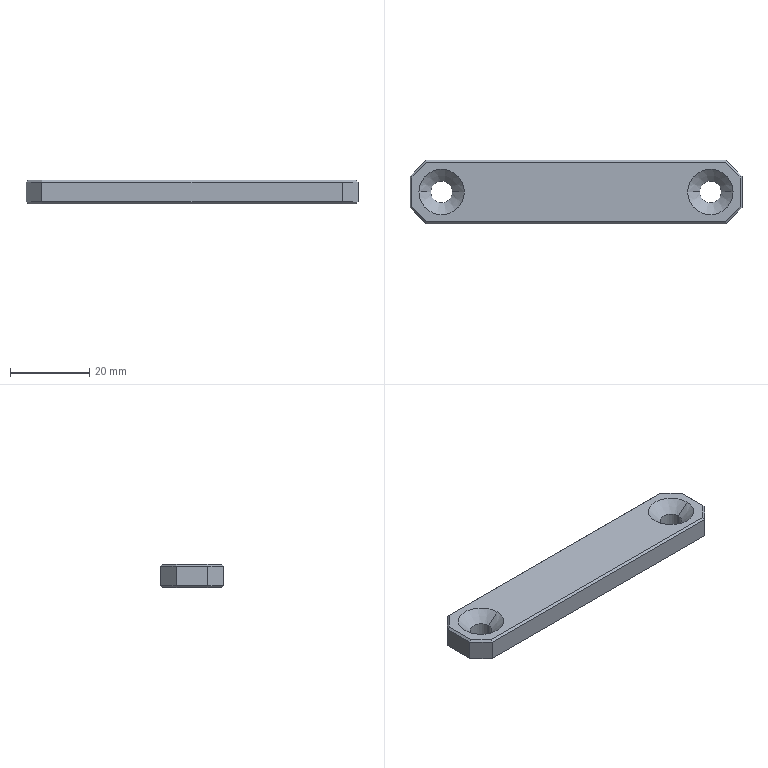Part | Creo | 1 solid | 34 faces | box 84 x 16 x 5.998 mm | volume 7341 mm3 | plane 26 | cylinder 4 | cone 4 | commonest cylinder face diameters 5.5 x4
STEP:
#1=CARTESIAN_POINT('',(-206.793,218.496,285.));
#2=VERTEX_POINT('',#1);
#3=CARTESIAN_POINT('',(-210.5,214.789,285.));
#4=VERTEX_POINT('',#3);
#5=CARTESIAN_POINT('',(-206.793,218.496,285.));
#6=DIRECTION('',(-0.7071,-0.7071,0.));
#7=VECTOR('',#6,5.243);
#8=LINE('',#5,#7);
#9=EDGE_CURVE('',#2,#4,#8,.T.);
#10=ORIENTED_EDGE('',*,*,#9,.F.);
#11=CARTESIAN_POINT('',(-131.207,218.496,285.));
#12=VERTEX_POINT('',#11);
#13=CARTESIAN_POINT('',(-206.793,218.496,285.));
#14=DIRECTION('',(1.,0.,0.));
#15=VECTOR('',#14,75.586);
#16=LINE('',#13,#15);
#17=EDGE_CURVE('',#2,#12,#16,.T.);
#18=ORIENTED_EDGE('',*,*,#17,.T.);
#19=CARTESIAN_POINT('',(-127.5,214.789,285.));
#20=VERTEX_POINT('',#19);
#21=CARTESIAN_POINT('',(-127.5,214.789,285.));
#22=DIRECTION('',(-0.7071,0.7071,0.));
#23=VECTOR('',#22,5.243);
#24=LINE('',#21,#23);
#25=EDGE_CURVE('',#20,#12,#24,.T.);
#26=ORIENTED_EDGE('',*,*,#25,.F.);
#27=CARTESIAN_POINT('',(-127.5,207.203,285.));
#28=VERTEX_POINT('',#27);
#29=CARTESIAN_POINT('',(-127.5,214.789,285.));
#30=DIRECTION('',(0.,-1.,0.));
#31=VECTOR('',#30,7.586);
#32=LINE('',#29,#31);
#33=EDGE_CURVE('',#20,#28,#32,.T.);
#34=ORIENTED_EDGE('',*,*,#33,.T.);
#35=CARTESIAN_POINT('',(-131.207,203.496,285.));
#36=VERTEX_POINT('',#35);
#37=CARTESIAN_POINT('',(-131.207,203.496,285.));
#38=DIRECTION('',(0.7071,0.7071,0.));
#39=VECTOR('',#38,5.243);
#40=LINE('',#37,#39);
#41=EDGE_CURVE('',#36,#28,#40,.T.);
#42=ORIENTED_EDGE('',*,*,#41,.F.);
#43=CARTESIAN_POINT('',(-206.793,203.496,285.));
#44=VERTEX_POINT('',#43);
#45=CARTESIAN_POINT('',(-131.207,203.496,285.));
#46=DIRECTION('',(-1.,0.,0.));
#47=VECTOR('',#46,75.586);
#48=LINE('',#45,#47);
#49=EDGE_CURVE('',#36,#44,#48,.T.);
#50=ORIENTED_EDGE('',*,*,#49,.T.);
#51=CARTESIAN_POINT('',(-210.5,207.203,285.));
#52=VERTEX_POINT('',#51);
#53=CARTESIAN_POINT('',(-210.5,207.203,285.));
#54=DIRECTION('',(0.7071,-0.7071,0.));
#55=VECTOR('',#54,5.243);
#56=LINE('',#53,#55);
#57=EDGE_CURVE('',#52,#44,#56,.T.);
#58=ORIENTED_EDGE('',*,*,#57,.F.);
#59=CARTESIAN_POINT('',(-210.5,207.203,285.));
#60=DIRECTION('',(0.,1.,0.));
#61=VECTOR('',#60,7.586);
#62=LINE('',#59,#61);
#63=EDGE_CURVE('',#52,#4,#62,.T.);
#64=ORIENTED_EDGE('',*,*,#63,.T.);
#65=EDGE_LOOP('',(#10,#18,#26,#34,#42,#50,#58,#64));
#66=FACE_OUTER_BOUND('',#65,.F.);
#67=CARTESIAN_POINT('',(-129.25,210.996,285.));
#68=VERTEX_POINT('',#67);
#69=CARTESIAN_POINT('',(-140.75,210.996,285.));
#70=VERTEX_POINT('',#69);
#71=CARTESIAN_POINT('',(-135.,210.996,285.));
#72=DIRECTION('',(0.,0.,-1.));
#73=DIRECTION('',(1.,0.,0.));
#74=AXIS2_PLACEMENT_3D('',#71,#72,#73);
#75=CIRCLE('',#74,5.75);
#76=EDGE_CURVE('',#68,#70,#75,.T.);
#77=ORIENTED_EDGE('',*,*,#76,.F.);
#78=CARTESIAN_POINT('',(-135.,210.996,285.));
#79=DIRECTION('',(0.,0.,-1.));
#80=DIRECTION('',(-1.,0.,0.));
#81=AXIS2_PLACEMENT_3D('',#78,#79,#80);
#82=CIRCLE('',#81,5.75);
#83=EDGE_CURVE('',#70,#68,#82,.T.);
#84=ORIENTED_EDGE('',*,*,#83,.F.);
#85=EDGE_LOOP('',(#77,#84));
#86=FACE_BOUND('',#85,.F.);
#87=CARTESIAN_POINT('',(-197.25,210.996,285.));
#88=VERTEX_POINT('',#87);
#89=CARTESIAN_POINT('',(-208.75,210.996,285.));
#90=VERTEX_POINT('',#89);
#91=CARTESIAN_POINT('',(-203.,210.996,285.));
#92=DIRECTION('',(0.,0.,-1.));
#93=DIRECTION('',(1.,0.,0.));
#94=AXIS2_PLACEMENT_3D('',#91,#92,#93);
#95=CIRCLE('',#94,5.75);
#96=EDGE_CURVE('',#88,#90,#95,.T.);
#97=ORIENTED_EDGE('',*,*,#96,.F.);
#98=CARTESIAN_POINT('',(-203.,210.996,285.));
#99=DIRECTION('',(0.,0.,-1.));
#100=DIRECTION('',(-1.,0.,0.));
#101=AXIS2_PLACEMENT_3D('',#98,#99,#100);
#102=CIRCLE('',#101,5.75);
#103=EDGE_CURVE('',#90,#88,#102,.T.);
#104=ORIENTED_EDGE('',*,*,#103,.F.);
#105=EDGE_LOOP('',(#97,#104));
#106=FACE_BOUND('',#105,.F.);
#107=CARTESIAN_POINT('',(6311.778,141.56,285.));
#108=DIRECTION('',(0.,0.,1.));
#109=DIRECTION('',(1.,0.,0.));
#110=AXIS2_PLACEMENT_3D('',#107,#108,#109);
#111=PLANE('',#110);
#112=ADVANCED_FACE('',(#66,#86,#106),#111,.T.);
#113=CARTESIAN_POINT('',(-207.,218.996,284.5));
#114=VERTEX_POINT('',#113);
#115=CARTESIAN_POINT('',(-207.,218.996,284.5));
#116=DIRECTION('',(0.2811,-0.6786,0.6786));
#117=VECTOR('',#116,0.7368);
#118=LINE('',#115,#117);
#119=EDGE_CURVE('',#114,#2,#118,.T.);
#120=ORIENTED_EDGE('',*,*,#119,.T.);
#121=ORIENTED_EDGE('',*,*,#9,.T.);
#122=CARTESIAN_POINT('',(-211.,214.996,284.5));
#123=VERTEX_POINT('',#122);
#124=CARTESIAN_POINT('',(-210.5,214.789,285.));
#125=DIRECTION('',(-0.6786,0.2811,-0.6786));
#126=VECTOR('',#125,0.7368);
#127=LINE('',#124,#126);
#128=EDGE_CURVE('',#4,#123,#127,.T.);
#129=ORIENTED_EDGE('',*,*,#128,.T.);
#130=CARTESIAN_POINT('',(-207.,218.996,284.5));
#131=DIRECTION('',(-0.7071,-0.7071,0.));
#132=VECTOR('',#131,5.657);
#133=LINE('',#130,#132);
#134=EDGE_CURVE('',#114,#123,#133,.T.);
#135=ORIENTED_EDGE('',*,*,#134,.F.);
#136=EDGE_LOOP('',(#120,#121,#129,#135));
#137=FACE_OUTER_BOUND('',#136,.F.);
#138=CARTESIAN_POINT('',(3014.025,3439.313,285.));
#139=DIRECTION('',(-0.5,0.5,0.7071));
#140=DIRECTION('',(0.7071,0.7071,0.));
#141=AXIS2_PLACEMENT_3D('',#138,#139,#140);
#142=PLANE('',#141);
#143=ADVANCED_FACE('',(#137),#142,.T.);
#144=CARTESIAN_POINT('',(-131.,218.996,284.5));
#145=VERTEX_POINT('',#144);
#146=CARTESIAN_POINT('',(-131.,218.996,284.5));
#147=DIRECTION('',(-0.2811,-0.6786,0.6786));
#148=VECTOR('',#147,0.7368);
#149=LINE('',#146,#148);
#150=EDGE_CURVE('',#145,#12,#149,.T.);
#151=ORIENTED_EDGE('',*,*,#150,.T.);
#152=ORIENTED_EDGE('',*,*,#17,.F.);
#153=ORIENTED_EDGE('',*,*,#119,.F.);
#154=CARTESIAN_POINT('',(-131.,218.996,284.5));
#155=DIRECTION('',(-1.,0.,0.));
#156=VECTOR('',#155,76.);
#157=LINE('',#154,#156);
#158=EDGE_CURVE('',#145,#114,#157,.T.);
#159=ORIENTED_EDGE('',*,*,#158,.F.);
#160=EDGE_LOOP('',(#151,#152,#153,#159));
#161=FACE_OUTER_BOUND('',#160,.F.);
#162=CARTESIAN_POINT('',(-160.,218.996,284.5));
#163=DIRECTION('',(0.,-0.7071,-0.7071));
#164=DIRECTION('',(1.,0.,0.));
#165=AXIS2_PLACEMENT_3D('',#162,#163,#164);
#166=PLANE('',#165);
#167=ADVANCED_FACE('',(#161),#166,.F.);
#168=CARTESIAN_POINT('',(-127.,214.996,284.5));
#169=VERTEX_POINT('',#168);
#170=CARTESIAN_POINT('',(-127.,214.996,284.5));
#171=DIRECTION('',(-0.6786,-0.2811,0.6786));
#172=VECTOR('',#171,0.7368);
#173=LINE('',#170,#172);
#174=EDGE_CURVE('',#169,#20,#173,.T.);
#175=ORIENTED_EDGE('',*,*,#174,.T.);
#176=ORIENTED_EDGE('',*,*,#25,.T.);
#177=ORIENTED_EDGE('',*,*,#150,.F.);
#178=CARTESIAN_POINT('',(-127.,214.996,284.5));
#179=DIRECTION('',(-0.7071,0.7071,0.));
#180=VECTOR('',#179,5.657);
#181=LINE('',#178,#180);
#182=EDGE_CURVE('',#169,#145,#181,.T.);
#183=ORIENTED_EDGE('',*,*,#182,.F.);
#184=EDGE_LOOP('',(#175,#176,#177,#183));
#185=FACE_OUTER_BOUND('',#184,.F.);
#186=CARTESIAN_POINT('',(3128.753,-3041.464,285.));
#187=DIRECTION('',(0.5,0.5,0.7071));
#188=DIRECTION('',(0.7071,-0.7071,0.));
#189=AXIS2_PLACEMENT_3D('',#186,#187,#188);
#190=PLANE('',#189);
#191=ADVANCED_FACE('',(#185),#190,.T.);
#192=CARTESIAN_POINT('',(-127.,206.996,284.5));
#193=VERTEX_POINT('',#192);
#194=CARTESIAN_POINT('',(-127.,206.996,284.5));
#195=DIRECTION('',(-0.6786,0.2811,0.6786));
#196=VECTOR('',#195,0.7368);
#197=LINE('',#194,#196);
#198=EDGE_CURVE('',#193,#28,#197,.T.);
#199=ORIENTED_EDGE('',*,*,#198,.T.);
#200=ORIENTED_EDGE('',*,*,#33,.F.);
#201=ORIENTED_EDGE('',*,*,#174,.F.);
#202=CARTESIAN_POINT('',(-127.,206.996,284.5));
#203=DIRECTION('',(0.,1.,0.));
#204=VECTOR('',#203,8.);
#205=LINE('',#202,#204);
#206=EDGE_CURVE('',#193,#169,#205,.T.);
#207=ORIENTED_EDGE('',*,*,#206,.F.);
#208=EDGE_LOOP('',(#199,#200,#201,#207));
#209=FACE_OUTER_BOUND('',#208,.F.);
#210=CARTESIAN_POINT('',(-127.,210.996,284.5));
#211=DIRECTION('',(-0.7071,0.,-0.7071));
#212=DIRECTION('',(0.,-1.,0.));
#213=AXIS2_PLACEMENT_3D('',#210,#211,#212);
#214=PLANE('',#213);
#215=ADVANCED_FACE('',(#209),#214,.F.);
#216=CARTESIAN_POINT('',(-131.,202.996,284.5));
#217=VERTEX_POINT('',#216);
#218=CARTESIAN_POINT('',(-131.207,203.496,285.));
#219=DIRECTION('',(0.2811,-0.6786,-0.6786));
#220=VECTOR('',#219,0.7368);
#221=LINE('',#218,#220);
#222=EDGE_CURVE('',#36,#217,#221,.T.);
#223=ORIENTED_EDGE('',*,*,#222,.F.);
#224=ORIENTED_EDGE('',*,*,#41,.T.);
#225=ORIENTED_EDGE('',*,*,#198,.F.);
#226=CARTESIAN_POINT('',(-131.,202.996,284.5));
#227=DIRECTION('',(0.7071,0.7071,0.));
#228=VECTOR('',#227,5.657);
#229=LINE('',#226,#228);
#230=EDGE_CURVE('',#217,#193,#229,.T.);
#231=ORIENTED_EDGE('',*,*,#230,.F.);
#232=EDGE_LOOP('',(#223,#224,#225,#231));
#233=FACE_OUTER_BOUND('',#232,.F.);
#234=CARTESIAN_POINT('',(3059.317,3394.021,285.));
#235=DIRECTION('',(0.5,-0.5,0.7071));
#236=DIRECTION('',(-0.7071,-0.7071,0.));
#237=AXIS2_PLACEMENT_3D('',#234,#235,#236);
#238=PLANE('',#237);
#239=ADVANCED_FACE('',(#233),#238,.T.);
#240=ORIENTED_EDGE('',*,*,#222,.T.);
#241=CARTESIAN_POINT('',(-207.,202.996,284.5));
#242=VERTEX_POINT('',#241);
#243=CARTESIAN_POINT('',(-207.,202.996,284.5));
#244=DIRECTION('',(1.,0.,0.));
#245=VECTOR('',#244,76.);
#246=LINE('',#243,#245);
#247=EDGE_CURVE('',#242,#217,#246,.T.);
#248=ORIENTED_EDGE('',*,*,#247,.F.);
#249=CARTESIAN_POINT('',(-206.793,203.496,285.));
#250=DIRECTION('',(-0.2811,-0.6786,-0.6786));
#251=VECTOR('',#250,0.7368);
#252=LINE('',#249,#251);
#253=EDGE_CURVE('',#44,#242,#252,.T.);
#254=ORIENTED_EDGE('',*,*,#253,.F.);
#255=ORIENTED_EDGE('',*,*,#49,.F.);
#256=EDGE_LOOP('',(#240,#248,#254,#255));
#257=FACE_OUTER_BOUND('',#256,.F.);
#258=CARTESIAN_POINT('',(-160.,202.996,284.5));
#259=DIRECTION('',(0.,0.7071,-0.7071));
#260=DIRECTION('',(-1.,0.,0.));
#261=AXIS2_PLACEMENT_3D('',#258,#259,#260);
#262=PLANE('',#261);
#263=ADVANCED_FACE('',(#257),#262,.F.);
#264=CARTESIAN_POINT('',(-207.,202.996,279.502));
#265=VERTEX_POINT('',#264);
#266=CARTESIAN_POINT('',(-207.,202.996,279.502));
#267=DIRECTION('',(0.,0.,1.));
#268=VECTOR('',#267,4.998);
#269=LINE('',#266,#268);
#270=EDGE_CURVE('',#265,#242,#269,.T.);
#271=ORIENTED_EDGE('',*,*,#270,.T.);
#272=ORIENTED_EDGE('',*,*,#247,.T.);
#273=CARTESIAN_POINT('',(-131.,202.996,279.502));
#274=VERTEX_POINT('',#273);
#275=CARTESIAN_POINT('',(-131.,202.996,284.5));
#276=DIRECTION('',(0.,0.,-1.));
#277=VECTOR('',#276,4.998);
#278=LINE('',#275,#277);
#279=EDGE_CURVE('',#217,#274,#278,.T.);
#280=ORIENTED_EDGE('',*,*,#279,.T.);
#281=CARTESIAN_POINT('',(-131.,202.996,279.502));
#282=DIRECTION('',(-1.,0.,0.));
#283=VECTOR('',#282,76.);
#284=LINE('',#281,#283);
#285=EDGE_CURVE('',#274,#265,#284,.T.);
#286=ORIENTED_EDGE('',*,*,#285,.T.);
#287=EDGE_LOOP('',(#271,#272,#280,#286));
#288=FACE_OUTER_BOUND('',#287,.F.);
#289=CARTESIAN_POINT('',(-160.,202.996,276.002));
#290=DIRECTION('',(0.,-1.,0.));
#291=DIRECTION('',(0.,0.,-1.));
#292=AXIS2_PLACEMENT_3D('',#289,#290,#291);
#293=PLANE('',#292);
#294=ADVANCED_FACE('',(#288),#293,.T.);
#295=ORIENTED_EDGE('',*,*,#270,.F.);
#296=CARTESIAN_POINT('',(-211.,206.996,279.502));
#297=VERTEX_POINT('',#296);
#298=CARTESIAN_POINT('',(-207.,202.996,279.502));
#299=DIRECTION('',(-0.7071,0.7071,0.));
#300=VECTOR('',#299,5.657);
#301=LINE('',#298,#300);
#302=EDGE_CURVE('',#265,#297,#301,.T.);
#303=ORIENTED_EDGE('',*,*,#302,.T.);
#304=CARTESIAN_POINT('',(-211.,206.996,284.5));
#305=VERTEX_POINT('',#304);
#306=CARTESIAN_POINT('',(-211.,206.996,284.5));
#307=DIRECTION('',(0.,0.,-1.));
#308=VECTOR('',#307,4.998);
#309=LINE('',#306,#308);
#310=EDGE_CURVE('',#305,#297,#309,.T.);
#311=ORIENTED_EDGE('',*,*,#310,.F.);
#312=CARTESIAN_POINT('',(-211.,206.996,284.5));
#313=DIRECTION('',(0.7071,-0.7071,0.));
#314=VECTOR('',#313,5.657);
#315=LINE('',#312,#314);
#316=EDGE_CURVE('',#305,#242,#315,.T.);
#317=ORIENTED_EDGE('',*,*,#316,.T.);
#318=EDGE_LOOP('',(#295,#303,#311,#317));
#319=FACE_OUTER_BOUND('',#318,.F.);
#320=CARTESIAN_POINT('',(-211.,206.996,276.002));
#321=DIRECTION('',(0.7071,0.7071,0.));
#322=DIRECTION('',(0.,0.,1.));
#323=AXIS2_PLACEMENT_3D('',#320,#321,#322);
#324=PLANE('',#323);
#325=ADVANCED_FACE('',(#319),#324,.F.);
#326=CARTESIAN_POINT('',(-206.793,203.496,279.002));
#327=VERTEX_POINT('',#326);
#328=CARTESIAN_POINT('',(-207.,202.996,279.502));
#329=DIRECTION('',(0.2811,0.6786,-0.6786));
#330=VECTOR('',#329,0.7368);
#331=LINE('',#328,#330);
#332=EDGE_CURVE('',#265,#327,#331,.T.);
#333=ORIENTED_EDGE('',*,*,#332,.T.);
#334=CARTESIAN_POINT('',(-210.5,207.203,279.002));
#335=VERTEX_POINT('',#334);
#336=CARTESIAN_POINT('',(-206.793,203.496,279.002));
#337=DIRECTION('',(-0.7071,0.7071,0.));
#338=VECTOR('',#337,5.243);
#339=LINE('',#336,#338);
#340=EDGE_CURVE('',#327,#335,#339,.T.);
#341=ORIENTED_EDGE('',*,*,#340,.T.);
#342=CARTESIAN_POINT('',(-211.,206.996,279.502));
#343=DIRECTION('',(0.6786,0.2811,-0.6786));
#344=VECTOR('',#343,0.7368);
#345=LINE('',#342,#344);
#346=EDGE_CURVE('',#297,#335,#345,.T.);
#347=ORIENTED_EDGE('',*,*,#346,.F.);
#348=ORIENTED_EDGE('',*,*,#302,.F.);
#349=EDGE_LOOP('',(#333,#341,#347,#348));
#350=FACE_OUTER_BOUND('',#349,.F.);
#351=CARTESIAN_POINT('',(-174.646,171.35,279.002));
#352=DIRECTION('',(0.5,0.5,0.7071));
#353=DIRECTION('',(-0.7071,0.7071,0.));
#354=AXIS2_PLACEMENT_3D('',#351,#352,#353);
#355=PLANE('',#354);
#356=ADVANCED_FACE('',(#350),#355,.F.);
#357=CARTESIAN_POINT('',(-131.207,203.496,279.002));
#358=VERTEX_POINT('',#357);
#359=CARTESIAN_POINT('',(-131.,202.996,279.502));
#360=DIRECTION('',(-0.2811,0.6786,-0.6786));
#361=VECTOR('',#360,0.7368);
#362=LINE('',#359,#361);
#363=EDGE_CURVE('',#274,#358,#362,.T.);
#364=ORIENTED_EDGE('',*,*,#363,.T.);
#365=CARTESIAN_POINT('',(-206.793,203.496,279.002));
#366=DIRECTION('',(1.,0.,0.));
#367=VECTOR('',#366,75.586);
#368=LINE('',#365,#367);
#369=EDGE_CURVE('',#327,#358,#368,.T.);
#370=ORIENTED_EDGE('',*,*,#369,.F.);
#371=ORIENTED_EDGE('',*,*,#332,.F.);
#372=ORIENTED_EDGE('',*,*,#285,.F.);
#373=EDGE_LOOP('',(#364,#370,#371,#372));
#374=FACE_OUTER_BOUND('',#373,.F.);
#375=CARTESIAN_POINT('',(-160.,202.996,279.502));
#376=DIRECTION('',(0.,-0.7071,-0.7071));
#377=DIRECTION('',(-1.,0.,0.));
#378=AXIS2_PLACEMENT_3D('',#375,#376,#377);
#379=PLANE('',#378);
#380=ADVANCED_FACE('',(#374),#379,.T.);
#381=CARTESIAN_POINT('',(-127.5,207.203,279.002));
#382=VERTEX_POINT('',#381);
#383=CARTESIAN_POINT('',(-127.,206.996,279.502));
#384=VERTEX_POINT('',#383);
#385=CARTESIAN_POINT('',(-127.5,207.203,279.002));
#386=DIRECTION('',(0.6786,-0.2811,0.6786));
#387=VECTOR('',#386,0.7368);
#388=LINE('',#385,#387);
#389=EDGE_CURVE('',#382,#384,#388,.T.);
#390=ORIENTED_EDGE('',*,*,#389,.F.);
#391=CARTESIAN_POINT('',(-127.5,207.203,279.002));
#392=DIRECTION('',(-0.7071,-0.7071,0.));
#393=VECTOR('',#392,5.243);
#394=LINE('',#391,#393);
#395=EDGE_CURVE('',#382,#358,#394,.T.);
#396=ORIENTED_EDGE('',*,*,#395,.T.);
#397=ORIENTED_EDGE('',*,*,#363,.F.);
#398=CARTESIAN_POINT('',(-127.,206.996,279.502));
#399=DIRECTION('',(-0.7071,-0.7071,0.));
#400=VECTOR('',#399,5.657);
#401=LINE('',#398,#400);
#402=EDGE_CURVE('',#384,#274,#401,.T.);
#403=ORIENTED_EDGE('',*,*,#402,.F.);
#404=EDGE_LOOP('',(#390,#396,#397,#403));
#405=FACE_OUTER_BOUND('',#404,.F.);
#406=CARTESIAN_POINT('',(-129.354,205.35,279.002));
#407=DIRECTION('',(-0.5,0.5,0.7071));
#408=DIRECTION('',(-0.7071,-0.7071,0.));
#409=AXIS2_PLACEMENT_3D('',#406,#407,#408);
#410=PLANE('',#409);
#411=ADVANCED_FACE('',(#405),#410,.F.);
#412=ORIENTED_EDGE('',*,*,#389,.T.);
#413=CARTESIAN_POINT('',(-127.,214.996,279.502));
#414=VERTEX_POINT('',#413);
#415=CARTESIAN_POINT('',(-127.,214.996,279.502));
#416=DIRECTION('',(0.,-1.,0.));
#417=VECTOR('',#416,8.);
#418=LINE('',#415,#417);
#419=EDGE_CURVE('',#414,#384,#418,.T.);
#420=ORIENTED_EDGE('',*,*,#419,.F.);
#421=CARTESIAN_POINT('',(-127.5,214.789,279.002));
#422=VERTEX_POINT('',#421);
#423=CARTESIAN_POINT('',(-127.5,214.789,279.002));
#424=DIRECTION('',(0.6786,0.2811,0.6786));
#425=VECTOR('',#424,0.7368);
#426=LINE('',#423,#425);
#427=EDGE_CURVE('',#422,#414,#426,.T.);
#428=ORIENTED_EDGE('',*,*,#427,.F.);
#429=CARTESIAN_POINT('',(-127.5,207.203,279.002));
#430=DIRECTION('',(0.,1.,0.));
#431=VECTOR('',#430,7.586);
#432=LINE('',#429,#431);
#433=EDGE_CURVE('',#382,#422,#432,.T.);
#434=ORIENTED_EDGE('',*,*,#433,.F.);
#435=EDGE_LOOP('',(#412,#420,#428,#434));
#436=FACE_OUTER_BOUND('',#435,.F.);
#437=CARTESIAN_POINT('',(-127.,210.996,279.502));
#438=DIRECTION('',(0.7071,0.,-0.7071));
#439=DIRECTION('',(0.,-1.,0.));
#440=AXIS2_PLACEMENT_3D('',#437,#438,#439);
#441=PLANE('',#440);
#442=ADVANCED_FACE('',(#436),#441,.T.);
#443=CARTESIAN_POINT('',(-127.,206.996,279.502));
#444=DIRECTION('',(0.,0.,1.));
#445=VECTOR('',#444,4.998);
#446=LINE('',#443,#445);
#447=EDGE_CURVE('',#384,#193,#446,.T.);
#448=ORIENTED_EDGE('',*,*,#447,.T.);
#449=ORIENTED_EDGE('',*,*,#206,.T.);
#450=CARTESIAN_POINT('',(-127.,214.996,284.5));
#451=DIRECTION('',(0.,0.,-1.));
#452=VECTOR('',#451,4.998);
#453=LINE('',#450,#452);
#454=EDGE_CURVE('',#169,#414,#453,.T.);
#455=ORIENTED_EDGE('',*,*,#454,.T.);
#456=ORIENTED_EDGE('',*,*,#419,.T.);
#457=EDGE_LOOP('',(#448,#449,#455,#456));
#458=FACE_OUTER_BOUND('',#457,.F.);
#459=CARTESIAN_POINT('',(-127.,210.996,276.002));
#460=DIRECTION('',(1.,0.,0.));
#461=DIRECTION('',(0.,0.,-1.));
#462=AXIS2_PLACEMENT_3D('',#459,#460,#461);
#463=PLANE('',#462);
#464=ADVANCED_FACE('',(#458),#463,.T.);
#465=ORIENTED_EDGE('',*,*,#279,.F.);
#466=ORIENTED_EDGE('',*,*,#230,.T.);
#467=ORIENTED_EDGE('',*,*,#447,.F.);
#468=ORIENTED_EDGE('',*,*,#402,.T.);
#469=EDGE_LOOP('',(#465,#466,#467,#468));
#470=FACE_OUTER_BOUND('',#469,.F.);
#471=CARTESIAN_POINT('',(-131.,202.996,276.002));
#472=DIRECTION('',(-0.7071,0.7071,0.));
#473=DIRECTION('',(0.,0.,1.));
#474=AXIS2_PLACEMENT_3D('',#471,#472,#473);
#475=PLANE('',#474);
#476=ADVANCED_FACE('',(#470),#475,.F.);
#477=ORIENTED_EDGE('',*,*,#454,.F.);
#478=ORIENTED_EDGE('',*,*,#182,.T.);
#479=CARTESIAN_POINT('',(-131.,218.996,279.502));
#480=VERTEX_POINT('',#479);
#481=CARTESIAN_POINT('',(-131.,218.996,279.502));
#482=DIRECTION('',(0.,0.,1.));
#483=VECTOR('',#482,4.998);
#484=LINE('',#481,#483);
#485=EDGE_CURVE('',#480,#145,#484,.T.);
#486=ORIENTED_EDGE('',*,*,#485,.F.);
#487=CARTESIAN_POINT('',(-131.,218.996,279.502));
#488=DIRECTION('',(0.7071,-0.7071,0.));
#489=VECTOR('',#488,5.657);
#490=LINE('',#487,#489);
#491=EDGE_CURVE('',#480,#414,#490,.T.);
#492=ORIENTED_EDGE('',*,*,#491,.T.);
#493=EDGE_LOOP('',(#477,#478,#486,#492));
#494=FACE_OUTER_BOUND('',#493,.F.);
#495=CARTESIAN_POINT('',(-127.,214.996,276.002));
#496=DIRECTION('',(-0.7071,-0.7071,0.));
#497=DIRECTION('',(0.,0.,1.));
#498=AXIS2_PLACEMENT_3D('',#495,#496,#497);
#499=PLANE('',#498);
#500=ADVANCED_FACE('',(#494),#499,.F.);
#501=ORIENTED_EDGE('',*,*,#485,.T.);
#502=ORIENTED_EDGE('',*,*,#158,.T.);
#503=CARTESIAN_POINT('',(-207.,218.996,279.502));
#504=VERTEX_POINT('',#503);
#505=CARTESIAN_POINT('',(-207.,218.996,284.5));
#506=DIRECTION('',(0.,0.,-1.));
#507=VECTOR('',#506,4.998);
#508=LINE('',#505,#507);
#509=EDGE_CURVE('',#114,#504,#508,.T.);
#510=ORIENTED_EDGE('',*,*,#509,.T.);
#511=CARTESIAN_POINT('',(-207.,218.996,279.502));
#512=DIRECTION('',(1.,0.,0.));
#513=VECTOR('',#512,76.);
#514=LINE('',#511,#513);
#515=EDGE_CURVE('',#504,#480,#514,.T.);
#516=ORIENTED_EDGE('',*,*,#515,.T.);
#517=EDGE_LOOP('',(#501,#502,#510,#516));
#518=FACE_OUTER_BOUND('',#517,.F.);
#519=CARTESIAN_POINT('',(-160.,218.996,276.002));
#520=DIRECTION('',(0.,1.,0.));
#521=DIRECTION('',(0.,0.,1.));
#522=AXIS2_PLACEMENT_3D('',#519,#520,#521);
#523=PLANE('',#522);
#524=ADVANCED_FACE('',(#518),#523,.T.);
#525=CARTESIAN_POINT('',(-211.,214.996,279.502));
#526=VERTEX_POINT('',#525);
#527=CARTESIAN_POINT('',(-211.,214.996,279.502));
#528=DIRECTION('',(0.,0.,1.));
#529=VECTOR('',#528,4.998);
#530=LINE('',#527,#529);
#531=EDGE_CURVE('',#526,#123,#530,.T.);
#532=ORIENTED_EDGE('',*,*,#531,.F.);
#533=CARTESIAN_POINT('',(-211.,214.996,279.502));
#534=DIRECTION('',(0.7071,0.7071,0.));
#535=VECTOR('',#534,5.657);
#536=LINE('',#533,#535);
#537=EDGE_CURVE('',#526,#504,#536,.T.);
#538=ORIENTED_EDGE('',*,*,#537,.T.);
#539=ORIENTED_EDGE('',*,*,#509,.F.);
#540=ORIENTED_EDGE('',*,*,#134,.T.);
#541=EDGE_LOOP('',(#532,#538,#539,#540));
#542=FACE_OUTER_BOUND('',#541,.F.);
#543=CARTESIAN_POINT('',(-207.,218.996,276.002));
#544=DIRECTION('',(0.7071,-0.7071,0.));
#545=DIRECTION('',(0.,0.,1.));
#546=AXIS2_PLACEMENT_3D('',#543,#544,#545);
#547=PLANE('',#546);
#548=ADVANCED_FACE('',(#542),#547,.F.);
#549=ORIENTED_EDGE('',*,*,#531,.T.);
#550=CARTESIAN_POINT('',(-211.,214.996,284.5));
#551=DIRECTION('',(0.,-1.,0.));
#552=VECTOR('',#551,8.);
#553=LINE('',#550,#552);
#554=EDGE_CURVE('',#123,#305,#553,.T.);
#555=ORIENTED_EDGE('',*,*,#554,.T.);
#556=ORIENTED_EDGE('',*,*,#310,.T.);
#557=CARTESIAN_POINT('',(-211.,206.996,279.502));
#558=DIRECTION('',(0.,1.,0.));
#559=VECTOR('',#558,8.);
#560=LINE('',#557,#559);
#561=EDGE_CURVE('',#297,#526,#560,.T.);
#562=ORIENTED_EDGE('',*,*,#561,.T.);
#563=EDGE_LOOP('',(#549,#555,#556,#562));
#564=FACE_OUTER_BOUND('',#563,.F.);
#565=CARTESIAN_POINT('',(-211.,210.996,276.002));
#566=DIRECTION('',(-1.,0.,0.));
#567=DIRECTION('',(0.,0.,1.));
#568=AXIS2_PLACEMENT_3D('',#565,#566,#567);
#569=PLANE('',#568);
#570=ADVANCED_FACE('',(#564),#569,.T.);
#571=CARTESIAN_POINT('',(-210.5,207.203,285.));
#572=DIRECTION('',(-0.6786,-0.2811,-0.6786));
#573=VECTOR('',#572,0.7368);
#574=LINE('',#571,#573);
#575=EDGE_CURVE('',#52,#305,#574,.T.);
#576=ORIENTED_EDGE('',*,*,#575,.T.);
#577=ORIENTED_EDGE('',*,*,#554,.F.);
#578=ORIENTED_EDGE('',*,*,#128,.F.);
#579=ORIENTED_EDGE('',*,*,#63,.F.);
#580=EDGE_LOOP('',(#576,#577,#578,#579));
#581=FACE_OUTER_BOUND('',#580,.F.);
#582=CARTESIAN_POINT('',(-211.,210.996,284.5));
#583=DIRECTION('',(0.7071,0.,-0.7071));
#584=DIRECTION('',(0.,1.,0.));
#585=AXIS2_PLACEMENT_3D('',#582,#583,#584);
#586=PLANE('',#585);
#587=ADVANCED_FACE('',(#581),#586,.F.);
#588=ORIENTED_EDGE('',*,*,#253,.T.);
#589=ORIENTED_EDGE('',*,*,#316,.F.);
#590=ORIENTED_EDGE('',*,*,#575,.F.);
#591=ORIENTED_EDGE('',*,*,#57,.T.);
#592=EDGE_LOOP('',(#588,#589,#590,#591));
#593=FACE_OUTER_BOUND('',#592,.F.);
#594=CARTESIAN_POINT('',(3083.46,-3086.757,285.));
#595=DIRECTION('',(-0.5,-0.5,0.7071));
#596=DIRECTION('',(-0.7071,0.7071,0.));
#597=AXIS2_PLACEMENT_3D('',#594,#595,#596);
#598=PLANE('',#597);
#599=ADVANCED_FACE('',(#593),#598,.T.);
#600=ORIENTED_EDGE('',*,*,#346,.T.);
#601=CARTESIAN_POINT('',(-210.5,214.789,279.002));
#602=VERTEX_POINT('',#601);
#603=CARTESIAN_POINT('',(-210.5,214.789,279.002));
#604=DIRECTION('',(0.,-1.,0.));
#605=VECTOR('',#604,7.586);
#606=LINE('',#603,#605);
#607=EDGE_CURVE('',#602,#335,#606,.T.);
#608=ORIENTED_EDGE('',*,*,#607,.F.);
#609=CARTESIAN_POINT('',(-211.,214.996,279.502));
#610=DIRECTION('',(0.6786,-0.2811,-0.6786));
#611=VECTOR('',#610,0.7368);
#612=LINE('',#609,#611);
#613=EDGE_CURVE('',#526,#602,#612,.T.);
#614=ORIENTED_EDGE('',*,*,#613,.F.);
#615=ORIENTED_EDGE('',*,*,#561,.F.);
#616=EDGE_LOOP('',(#600,#608,#614,#615));
#617=FACE_OUTER_BOUND('',#616,.F.);
#618=CARTESIAN_POINT('',(-211.,210.996,279.502));
#619=DIRECTION('',(-0.7071,0.,-0.7071));
#620=DIRECTION('',(0.,1.,0.));
#621=AXIS2_PLACEMENT_3D('',#618,#619,#620);
#622=PLANE('',#621);
#623=ADVANCED_FACE('',(#617),#622,.T.);
#624=ORIENTED_EDGE('',*,*,#607,.T.);
#625=ORIENTED_EDGE('',*,*,#340,.F.);
#626=ORIENTED_EDGE('',*,*,#369,.T.);
#627=ORIENTED_EDGE('',*,*,#395,.F.);
#628=ORIENTED_EDGE('',*,*,#433,.T.);
#629=CARTESIAN_POINT('',(-131.207,218.496,279.002));
#630=VERTEX_POINT('',#629);
#631=CARTESIAN_POINT('',(-131.207,218.496,279.002));
#632=DIRECTION('',(0.7071,-0.7071,0.));
#633=VECTOR('',#632,5.243);
#634=LINE('',#631,#633);
#635=EDGE_CURVE('',#630,#422,#634,.T.);
#636=ORIENTED_EDGE('',*,*,#635,.F.);
#637=CARTESIAN_POINT('',(-206.793,218.496,279.002));
#638=VERTEX_POINT('',#637);
#639=CARTESIAN_POINT('',(-131.207,218.496,279.002));
#640=DIRECTION('',(-1.,0.,0.));
#641=VECTOR('',#640,75.586);
#642=LINE('',#639,#641);
#643=EDGE_CURVE('',#630,#638,#642,.T.);
#644=ORIENTED_EDGE('',*,*,#643,.T.);
#645=CARTESIAN_POINT('',(-210.5,214.789,279.002));
#646=DIRECTION('',(0.7071,0.7071,0.));
#647=VECTOR('',#646,5.243);
#648=LINE('',#645,#647);
#649=EDGE_CURVE('',#602,#638,#648,.T.);
#650=ORIENTED_EDGE('',*,*,#649,.F.);
#651=EDGE_LOOP('',(#624,#625,#626,#627,#628,#636,#644,#650));
#652=FACE_OUTER_BOUND('',#651,.F.);
#653=CARTESIAN_POINT('',(-132.25,210.996,279.002));
#654=VERTEX_POINT('',#653);
#655=CARTESIAN_POINT('',(-137.75,210.996,279.002));
#656=VERTEX_POINT('',#655);
#657=CARTESIAN_POINT('',(-135.,210.996,279.002));
#658=DIRECTION('',(0.,0.,1.));
#659=DIRECTION('',(1.,0.,0.));
#660=AXIS2_PLACEMENT_3D('',#657,#658,#659);
#661=CIRCLE('',#660,2.75);
#662=EDGE_CURVE('',#654,#656,#661,.T.);
#663=ORIENTED_EDGE('',*,*,#662,.F.);
#664=CARTESIAN_POINT('',(-135.,210.996,279.002));
#665=DIRECTION('',(0.,0.,1.));
#666=DIRECTION('',(-1.,0.,0.));
#667=AXIS2_PLACEMENT_3D('',#664,#665,#666);
#668=CIRCLE('',#667,2.75);
#669=EDGE_CURVE('',#656,#654,#668,.T.);
#670=ORIENTED_EDGE('',*,*,#669,.F.);
#671=EDGE_LOOP('',(#663,#670));
#672=FACE_BOUND('',#671,.F.);
#673=CARTESIAN_POINT('',(-200.25,210.996,279.002));
#674=VERTEX_POINT('',#673);
#675=CARTESIAN_POINT('',(-205.75,210.996,279.002));
#676=VERTEX_POINT('',#675);
#677=CARTESIAN_POINT('',(-203.,210.996,279.002));
#678=DIRECTION('',(0.,0.,1.));
#679=DIRECTION('',(1.,0.,0.));
#680=AXIS2_PLACEMENT_3D('',#677,#678,#679);
#681=CIRCLE('',#680,2.75);
#682=EDGE_CURVE('',#674,#676,#681,.T.);
#683=ORIENTED_EDGE('',*,*,#682,.F.);
#684=CARTESIAN_POINT('',(-203.,210.996,279.002));
#685=DIRECTION('',(0.,0.,1.));
#686=DIRECTION('',(-1.,0.,0.));
#687=AXIS2_PLACEMENT_3D('',#684,#685,#686);
#688=CIRCLE('',#687,2.75);
#689=EDGE_CURVE('',#676,#674,#688,.T.);
#690=ORIENTED_EDGE('',*,*,#689,.F.);
#691=EDGE_LOOP('',(#683,#690));
#692=FACE_BOUND('',#691,.F.);
#693=CARTESIAN_POINT('',(-135.,210.996,279.002));
#694=DIRECTION('',(0.,0.,1.));
#695=DIRECTION('',(1.,0.,0.));
#696=AXIS2_PLACEMENT_3D('',#693,#694,#695);
#697=PLANE('',#696);
#698=ADVANCED_FACE('',(#652,#672,#692),#697,.F.);
#699=ORIENTED_EDGE('',*,*,#427,.T.);
#700=ORIENTED_EDGE('',*,*,#491,.F.);
#701=CARTESIAN_POINT('',(-131.207,218.496,279.002));
#702=DIRECTION('',(0.2811,0.6786,0.6786));
#703=VECTOR('',#702,0.7368);
#704=LINE('',#701,#703);
#705=EDGE_CURVE('',#630,#480,#704,.T.);
#706=ORIENTED_EDGE('',*,*,#705,.F.);
#707=ORIENTED_EDGE('',*,*,#635,.T.);
#708=EDGE_LOOP('',(#699,#700,#706,#707));
#709=FACE_OUTER_BOUND('',#708,.F.);
#710=CARTESIAN_POINT('',(-129.354,216.642,279.002));
#711=DIRECTION('',(-0.5,-0.5,0.7071));
#712=DIRECTION('',(0.7071,-0.7071,0.));
#713=AXIS2_PLACEMENT_3D('',#710,#711,#712);
#714=PLANE('',#713);
#715=ADVANCED_FACE('',(#709),#714,.F.);
#716=ORIENTED_EDGE('',*,*,#705,.T.);
#717=ORIENTED_EDGE('',*,*,#515,.F.);
#718=CARTESIAN_POINT('',(-206.793,218.496,279.002));
#719=DIRECTION('',(-0.2811,0.6786,0.6786));
#720=VECTOR('',#719,0.7368);
#721=LINE('',#718,#720);
#722=EDGE_CURVE('',#638,#504,#721,.T.);
#723=ORIENTED_EDGE('',*,*,#722,.F.);
#724=ORIENTED_EDGE('',*,*,#643,.F.);
#725=EDGE_LOOP('',(#716,#717,#723,#724));
#726=FACE_OUTER_BOUND('',#725,.F.);
#727=CARTESIAN_POINT('',(-160.,218.996,279.502));
#728=DIRECTION('',(0.,0.7071,-0.7071));
#729=DIRECTION('',(1.,0.,0.));
#730=AXIS2_PLACEMENT_3D('',#727,#728,#729);
#731=PLANE('',#730);
#732=ADVANCED_FACE('',(#726),#731,.T.);
#733=ORIENTED_EDGE('',*,*,#613,.T.);
#734=ORIENTED_EDGE('',*,*,#649,.T.);
#735=ORIENTED_EDGE('',*,*,#722,.T.);
#736=ORIENTED_EDGE('',*,*,#537,.F.);
#737=EDGE_LOOP('',(#733,#734,#735,#736));
#738=FACE_OUTER_BOUND('',#737,.F.);
#739=CARTESIAN_POINT('',(-174.646,250.642,279.002));
#740=DIRECTION('',(0.5,-0.5,0.7071));
#741=DIRECTION('',(0.7071,0.7071,0.));
#742=AXIS2_PLACEMENT_3D('',#739,#740,#741);
#743=PLANE('',#742);
#744=ADVANCED_FACE('',(#738),#743,.F.);
#745=CARTESIAN_POINT('',(-137.75,210.996,282.231));
#746=VERTEX_POINT('',#745);
#747=CARTESIAN_POINT('',(-132.25,210.996,282.231));
#748=VERTEX_POINT('',#747);
#749=CARTESIAN_POINT('',(-135.,210.996,282.231));
#750=DIRECTION('',(0.,0.,-1.));
#751=DIRECTION('',(-1.,0.,0.));
#752=AXIS2_PLACEMENT_3D('',#749,#750,#751);
#753=CIRCLE('',#752,2.75);
#754=EDGE_CURVE('',#746,#748,#753,.T.);
#755=ORIENTED_EDGE('',*,*,#754,.T.);
#756=CARTESIAN_POINT('',(-132.25,210.996,279.002));
#757=DIRECTION('',(0.,0.,1.));
#758=VECTOR('',#757,3.229);
#759=LINE('',#756,#758);
#760=EDGE_CURVE('',#654,#748,#759,.T.);
#761=ORIENTED_EDGE('',*,*,#760,.F.);
#762=ORIENTED_EDGE('',*,*,#662,.T.);
#763=CARTESIAN_POINT('',(-137.75,210.996,279.002));
#764=DIRECTION('',(0.,0.,1.));
#765=VECTOR('',#764,3.229);
#766=LINE('',#763,#765);
#767=EDGE_CURVE('',#656,#746,#766,.T.);
#768=ORIENTED_EDGE('',*,*,#767,.T.);
#769=EDGE_LOOP('',(#755,#761,#762,#768));
#770=FACE_OUTER_BOUND('',#769,.F.);
#771=CARTESIAN_POINT('',(-135.,210.996,279.002));
#772=DIRECTION('',(0.,0.,1.));
#773=DIRECTION('',(1.,0.,0.));
#774=AXIS2_PLACEMENT_3D('',#771,#772,#773);
#775=CYLINDRICAL_SURFACE('',#774,2.75);
#776=ADVANCED_FACE('',(#770),#775,.F.);
#777=ORIENTED_EDGE('',*,*,#754,.F.);
#778=CARTESIAN_POINT('',(-137.75,210.996,282.231));
#779=DIRECTION('',(-0.7348,0.,0.6783));
#780=VECTOR('',#779,4.083);
#781=LINE('',#778,#780);
#782=EDGE_CURVE('',#746,#70,#781,.T.);
#783=ORIENTED_EDGE('',*,*,#782,.T.);
#784=ORIENTED_EDGE('',*,*,#83,.T.);
#785=CARTESIAN_POINT('',(-132.25,210.996,282.231));
#786=DIRECTION('',(0.7348,0.,0.6783));
#787=VECTOR('',#786,4.083);
#788=LINE('',#785,#787);
#789=EDGE_CURVE('',#748,#68,#788,.T.);
#790=ORIENTED_EDGE('',*,*,#789,.F.);
#791=EDGE_LOOP('',(#777,#783,#784,#790));
#792=FACE_OUTER_BOUND('',#791,.F.);
#793=CARTESIAN_POINT('',(-135.,210.996,283.615));
#794=DIRECTION('',(0.,0.,1.));
#795=DIRECTION('',(1.,0.,0.));
#796=AXIS2_PLACEMENT_3D('',#793,#794,#795);
#797=CONICAL_SURFACE('',#796,4.25,47.291);
#798=ADVANCED_FACE('',(#792),#797,.F.);
#799=CARTESIAN_POINT('',(-135.,210.996,282.231));
#800=DIRECTION('',(0.,0.,-1.));
#801=DIRECTION('',(1.,0.,0.));
#802=AXIS2_PLACEMENT_3D('',#799,#800,#801);
#803=CIRCLE('',#802,2.75);
#804=EDGE_CURVE('',#748,#746,#803,.T.);
#805=ORIENTED_EDGE('',*,*,#804,.F.);
#806=ORIENTED_EDGE('',*,*,#789,.T.);
#807=ORIENTED_EDGE('',*,*,#76,.T.);
#808=ORIENTED_EDGE('',*,*,#782,.F.);
#809=EDGE_LOOP('',(#805,#806,#807,#808));
#810=FACE_OUTER_BOUND('',#809,.F.);
#811=CARTESIAN_POINT('',(-135.,210.996,283.615));
#812=DIRECTION('',(0.,0.,1.));
#813=DIRECTION('',(1.,0.,0.));
#814=AXIS2_PLACEMENT_3D('',#811,#812,#813);
#815=CONICAL_SURFACE('',#814,4.25,47.291);
#816=ADVANCED_FACE('',(#810),#815,.F.);
#817=ORIENTED_EDGE('',*,*,#804,.T.);
#818=ORIENTED_EDGE('',*,*,#767,.F.);
#819=ORIENTED_EDGE('',*,*,#669,.T.);
#820=ORIENTED_EDGE('',*,*,#760,.T.);
#821=EDGE_LOOP('',(#817,#818,#819,#820));
#822=FACE_OUTER_BOUND('',#821,.F.);
#823=CARTESIAN_POINT('',(-135.,210.996,279.002));
#824=DIRECTION('',(0.,0.,1.));
#825=DIRECTION('',(1.,0.,0.));
#826=AXIS2_PLACEMENT_3D('',#823,#824,#825);
#827=CYLINDRICAL_SURFACE('',#826,2.75);
#828=ADVANCED_FACE('',(#822),#827,.F.);
#829=CARTESIAN_POINT('',(-205.75,210.996,282.231));
#830=VERTEX_POINT('',#829);
#831=CARTESIAN_POINT('',(-200.25,210.996,282.231));
#832=VERTEX_POINT('',#831);
#833=CARTESIAN_POINT('',(-203.,210.996,282.231));
#834=DIRECTION('',(0.,0.,-1.));
#835=DIRECTION('',(-1.,0.,0.));
#836=AXIS2_PLACEMENT_3D('',#833,#834,#835);
#837=CIRCLE('',#836,2.75);
#838=EDGE_CURVE('',#830,#832,#837,.T.);
#839=ORIENTED_EDGE('',*,*,#838,.T.);
#840=CARTESIAN_POINT('',(-200.25,210.996,279.002));
#841=DIRECTION('',(0.,0.,1.));
#842=VECTOR('',#841,3.229);
#843=LINE('',#840,#842);
#844=EDGE_CURVE('',#674,#832,#843,.T.);
#845=ORIENTED_EDGE('',*,*,#844,.F.);
#846=ORIENTED_EDGE('',*,*,#682,.T.);
#847=CARTESIAN_POINT('',(-205.75,210.996,279.002));
#848=DIRECTION('',(0.,0.,1.));
#849=VECTOR('',#848,3.229);
#850=LINE('',#847,#849);
#851=EDGE_CURVE('',#676,#830,#850,.T.);
#852=ORIENTED_EDGE('',*,*,#851,.T.);
#853=EDGE_LOOP('',(#839,#845,#846,#852));
#854=FACE_OUTER_BOUND('',#853,.F.);
#855=CARTESIAN_POINT('',(-203.,210.996,279.002));
#856=DIRECTION('',(0.,0.,1.));
#857=DIRECTION('',(1.,0.,0.));
#858=AXIS2_PLACEMENT_3D('',#855,#856,#857);
#859=CYLINDRICAL_SURFACE('',#858,2.75);
#860=ADVANCED_FACE('',(#854),#859,.F.);
#861=ORIENTED_EDGE('',*,*,#838,.F.);
#862=CARTESIAN_POINT('',(-205.75,210.996,282.231));
#863=DIRECTION('',(-0.7348,0.,0.6783));
#864=VECTOR('',#863,4.083);
#865=LINE('',#862,#864);
#866=EDGE_CURVE('',#830,#90,#865,.T.);
#867=ORIENTED_EDGE('',*,*,#866,.T.);
#868=ORIENTED_EDGE('',*,*,#103,.T.);
#869=CARTESIAN_POINT('',(-200.25,210.996,282.231));
#870=DIRECTION('',(0.7348,0.,0.6783));
#871=VECTOR('',#870,4.083);
#872=LINE('',#869,#871);
#873=EDGE_CURVE('',#832,#88,#872,.T.);
#874=ORIENTED_EDGE('',*,*,#873,.F.);
#875=EDGE_LOOP('',(#861,#867,#868,#874));
#876=FACE_OUTER_BOUND('',#875,.F.);
#877=CARTESIAN_POINT('',(-203.,210.996,283.615));
#878=DIRECTION('',(0.,0.,1.));
#879=DIRECTION('',(1.,0.,0.));
#880=AXIS2_PLACEMENT_3D('',#877,#878,#879);
#881=CONICAL_SURFACE('',#880,4.25,47.291);
#882=ADVANCED_FACE('',(#876),#881,.F.);
#883=CARTESIAN_POINT('',(-203.,210.996,282.231));
#884=DIRECTION('',(0.,0.,-1.));
#885=DIRECTION('',(1.,0.,0.));
#886=AXIS2_PLACEMENT_3D('',#883,#884,#885);
#887=CIRCLE('',#886,2.75);
#888=EDGE_CURVE('',#832,#830,#887,.T.);
#889=ORIENTED_EDGE('',*,*,#888,.F.);
#890=ORIENTED_EDGE('',*,*,#873,.T.);
#891=ORIENTED_EDGE('',*,*,#96,.T.);
#892=ORIENTED_EDGE('',*,*,#866,.F.);
#893=EDGE_LOOP('',(#889,#890,#891,#892));
#894=FACE_OUTER_BOUND('',#893,.F.);
#895=CARTESIAN_POINT('',(-203.,210.996,283.615));
#896=DIRECTION('',(0.,0.,1.));
#897=DIRECTION('',(1.,0.,0.));
#898=AXIS2_PLACEMENT_3D('',#895,#896,#897);
#899=CONICAL_SURFACE('',#898,4.25,47.291);
#900=ADVANCED_FACE('',(#894),#899,.F.);
#901=ORIENTED_EDGE('',*,*,#888,.T.);
#902=ORIENTED_EDGE('',*,*,#851,.F.);
#903=ORIENTED_EDGE('',*,*,#689,.T.);
#904=ORIENTED_EDGE('',*,*,#844,.T.);
#905=EDGE_LOOP('',(#901,#902,#903,#904));
#906=FACE_OUTER_BOUND('',#905,.F.);
#907=CARTESIAN_POINT('',(-203.,210.996,279.002));
#908=DIRECTION('',(0.,0.,1.));
#909=DIRECTION('',(1.,0.,0.));
#910=AXIS2_PLACEMENT_3D('',#907,#908,#909);
#911=CYLINDRICAL_SURFACE('',#910,2.75);
#912=ADVANCED_FACE('',(#906),#911,.F.);
#913=CLOSED_SHELL('',(#112,#143,#167,#191,#215,#239,#263,#294,#325,#356,#380,#411,#442,#464,#476,#500,#524,#548,#570,#587,#599,#623,#698,#715,#732,#744,#776,#798,#816,#828,#860,#882,#900,#912));
#914=MANIFOLD_SOLID_BREP('',#913);
#915=(LENGTH_UNIT()NAMED_UNIT(*)SI_UNIT(.MILLI.,.METRE.));
#916=UNCERTAINTY_MEASURE_WITH_UNIT(LENGTH_MEASURE(0.008572),#915,'','');
#917=(NAMED_UNIT(*)PLANE_ANGLE_UNIT()SI_UNIT($,.RADIAN.));
#918=PLANE_ANGLE_MEASURE_WITH_UNIT(PLANE_ANGLE_MEASURE(0.01745),#917);
#919=(CONVERSION_BASED_UNIT('DEGREE',#918)NAMED_UNIT(*)PLANE_ANGLE_UNIT());
#920=(NAMED_UNIT(*)SI_UNIT($,.STERADIAN.)SOLID_ANGLE_UNIT());
#921=(GEOMETRIC_REPRESENTATION_CONTEXT(3)GLOBAL_UNCERTAINTY_ASSIGNED_CONTEXT((#916))GLOBAL_UNIT_ASSIGNED_CONTEXT((#915,#919,#920))REPRESENTATION_CONTEXT('',''));
#922=ADVANCED_BREP_SHAPE_REPRESENTATION('',(#914),#921);